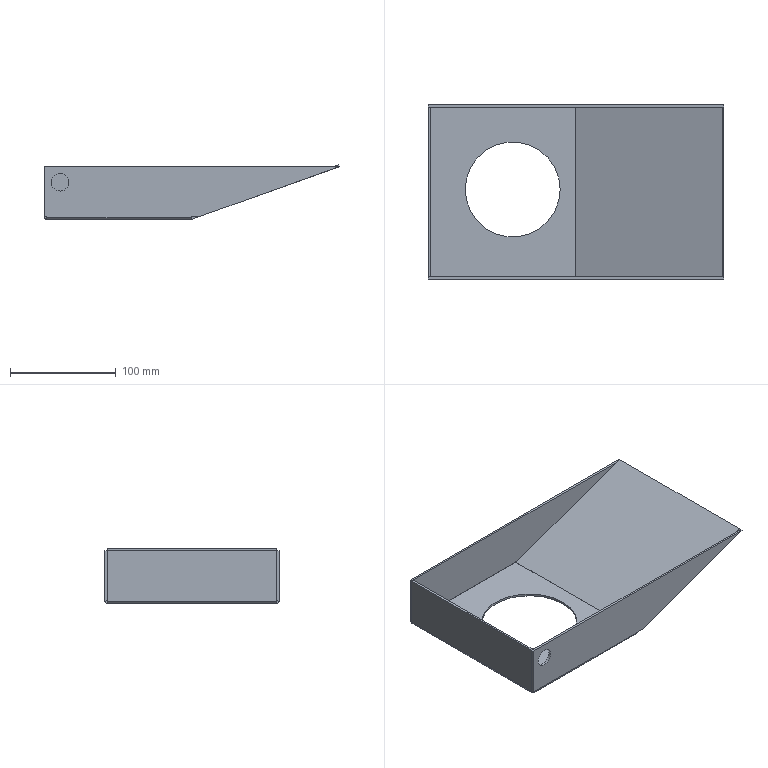Part | STEP file | Left Door Filler Piece A | 1 solid | 50 faces | box 280 x 165 x 51.682 mm | volume 136395 mm3 | plane 38 | cylinder 12 | commonest cylinder face diameters 0.2 x4 4.2 x4 16.5 x2 90 x2